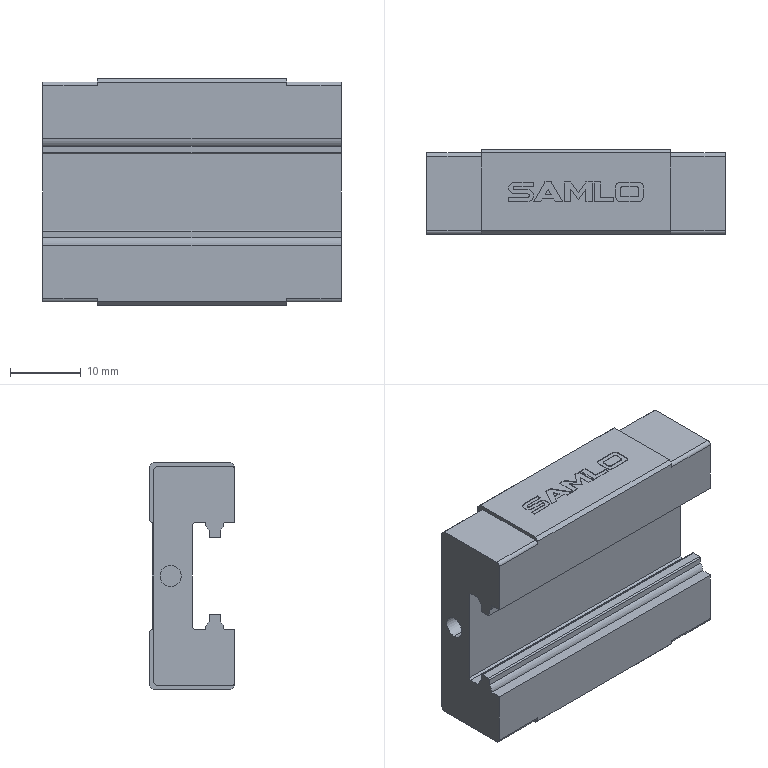Part | SolidWorks | features BaseBody 1 | 1 solid | 146 faces | box 42.1 x 12 x 32 mm | volume 11943 mm3 | plane 100 | cylinder 38 | cone 8 | commonest cylinder face diameters 2.459 x8 0.4 x4 0.643 x4 1 x4 1.363 x4 2.64 x4